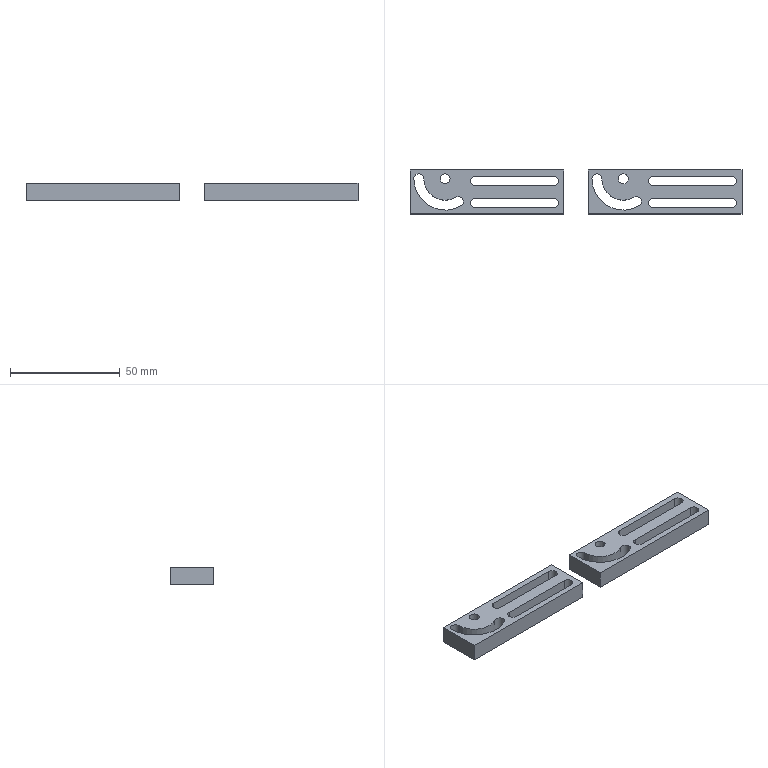CAM job | NX | 3-axis milling, drilling | part box 151 x 20 x 8 mm | stock box 156 x 25 x 10 mm
Tools:
number,name,description,diameter,corner_radius,flute_length,length,flutes
4,D4,平底铣刀-粗,4.0,0.0,25.0,75.0,2
9,D10,平底铣刀-粗,10.0,0.0,35.0,75.0,2
11,D4-J,平底铣刀-精,4.0,0.0,50.0,75.0,2
7,D6-J,平底铣刀-精,6.0,0.0,25.0,75.0,2
1,D80R0.8_FLYCUTTER,圆鼻刀-粗,80.0,0.8,50.0,75.0,2
1,D80R0.8_FLYCUTTER-J,圆鼻刀-精,80.0,0.8,50.0,75.0,2
2,D6_CHAMFER,倒角刀,6.0,0.0,3.0,25.0,2
11,ZT4.5,钻头,4.5,0.0,35.0,50.0,2
Operations:
program,operation,operation_type,tool,method,geometry_group,spindle_rpm,surface_speed,feed_per_tooth,feed_cut,feed_plunge,cut_length_mm,path_length_mm,cut_time_min,machine_time_min
B,FLOORWALL_FACEMILL_ONEPASS_ROUGH_COPY,VolumeBased25DMillingOperation,D80R0.8_FLYCUTTER,LAYERROUGH-DEPTHK-STEPG,W-B,2800.0,703.696,0.5357,3000.0,100.0,1036.776,1896.734,0.3456,0.4316
B,FLOORWALL_FACEMILL_ONEPASS_FINISH_COPY,VolumeBased25DMillingOperation,D80R0.8_FLYCUTTER-J,SIDEFINISH-DEPTHK-STEPG,W-B,4000.0,1005.28,0.125,1000.0,100.0,258.998,354.998,0.259,0.2686
B,PLANEDEBURR_6X45L_COPY,SurfaceContour,D6_CHAMFER,CLIMBCHAMFER-DEPTH0-STEPG,W-B,6500.0,122.519,0.1154,1500.0,100.0,857.05,1361.953,0.5714,0.6219
A,TOPFACE,FaceMilling,D80R0.8_FLYCUTTER,SIDEFINISH-DEPTHK-STEPG,W-A,4500.0,1385.0,0.1667,1500.0,100.0,245.0,341.0,0.1633,0.1729
A,PROFILEROUGH_2,VolumeBased25DMillingOperation,D10,METHOD,W-A,8000.0,251.327,0.375,6000.0,80.0,5092.093,5386.593,0.8487,0.8781
A,SPOT,Operation,D6_CHAMFER,METHOD,W-A,8000.0,150.796,0.1562,2500.0,0.0,5.0,192.006,0.002,0.0207
A,DRILLHOLE,Operation,ZT4.5,METHOD,W-A,3000.0,42.411,0.2,1200.0,0.0,23.704,229.414,0.0198,0.0403
A,THRUSLOTROUGH_1,VolumeBased25DMillingOperation,D4,METHOD,W-A,10000.0,125.664,0.06,1200.0,100.0,10365.777,10894.078,8.638,8.691
A,CORNERCLEAN_D4,ZLevelMilling,D4,METHOD,W-A,9000.0,113.097,0.1389,2500.0,80.0,2758.858,3053.658,1.104,1.133
A,SLOTFINISH_1,VolumeBased25DMillingOperation,D4-J,METHOD,W-A,8000.0,100.531,0.0312,500.0,100.0,598.393,1200.129,1.197,1.257
A,SLOTFINISH_2,VolumeBased25DMillingOperation,D4-J,METHOD,W-A,8000.0,100.531,0.05,800.0,100.0,216.272,547.831,0.2703,0.3035
A,BODYONLY,SurfaceContour,D6_CHAMFER,METHOD,W-A,8000.0,150.796,0.1875,3000.0,100.0,869.908,1679.447,0.29,0.3709
A,DRILLCHAMFER_1,Operation,D6_CHAMFER,METHOD,W-A,8000.0,150.796,0.0094,150.0,0.0,11.1,206.256,0.074,0.0935
A,PROFILESEMI_2,VolumeBased25DMillingOperation,D6-J,METHOD,W-A,9000.0,169.646,0.0556,1000.0,100.0,407.216,720.733,0.4072,0.4386